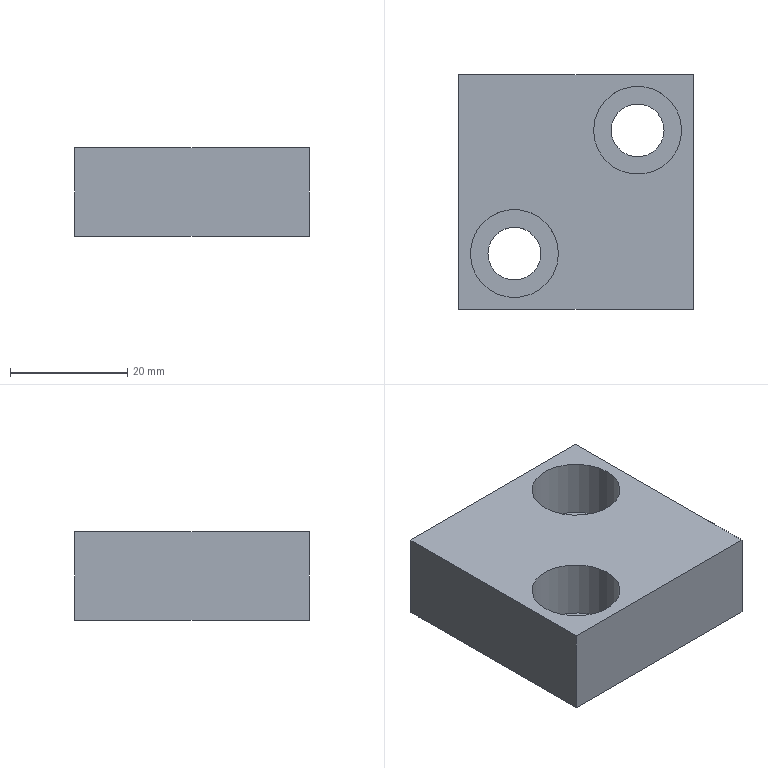Part | NX | features solid 2 | 1 solid | 12 faces | box 40 x 40 x 15 mm | volume 19830 mm3 | plane 8 | cylinder 4 | commonest cylinder face diameters 9 x2 15 x2
STEP:
#1=CARTESIAN_POINT('',(1490.,20.,251.));
#2=VERTEX_POINT('',#1);
#3=CARTESIAN_POINT('',(1490.,20.,266.));
#4=VERTEX_POINT('',#3);
#5=CARTESIAN_POINT('',(1490.,20.,251.));
#6=DIRECTION('',(0.,0.,1.));
#7=VECTOR('',#6,1000.);
#8=LINE('',#5,#7);
#9=EDGE_CURVE('',#2,#4,#8,.T.);
#10=ORIENTED_EDGE('',*,*,#9,.F.);
#11=CARTESIAN_POINT('',(1490.,60.,251.));
#12=VERTEX_POINT('',#11);
#13=CARTESIAN_POINT('',(1490.,60.,251.));
#14=DIRECTION('',(0.,-1.,0.));
#15=VECTOR('',#14,1000.);
#16=LINE('',#13,#15);
#17=EDGE_CURVE('',#12,#2,#16,.T.);
#18=ORIENTED_EDGE('',*,*,#17,.F.);
#19=CARTESIAN_POINT('',(1490.,60.,266.));
#20=VERTEX_POINT('',#19);
#21=CARTESIAN_POINT('',(1490.,60.,251.));
#22=DIRECTION('',(0.,0.,1.));
#23=VECTOR('',#22,1000.);
#24=LINE('',#21,#23);
#25=EDGE_CURVE('',#12,#20,#24,.T.);
#26=ORIENTED_EDGE('',*,*,#25,.T.);
#27=CARTESIAN_POINT('',(1490.,60.,266.));
#28=DIRECTION('',(0.,-1.,0.));
#29=VECTOR('',#28,1000.);
#30=LINE('',#27,#29);
#31=EDGE_CURVE('',#20,#4,#30,.T.);
#32=ORIENTED_EDGE('',*,*,#31,.T.);
#33=EDGE_LOOP('',(#10,#18,#26,#32));
#34=FACE_BOUND('',#33,.T.);
#35=CARTESIAN_POINT('',(1490.,60.,251.));
#36=DIRECTION('',(1.,0.,0.));
#37=DIRECTION('',(0.,0.,1.));
#38=AXIS2_PLACEMENT_3D('',#35,#36,#37);
#39=PLANE('',#38);
#40=ADVANCED_FACE('',(#34),#39,.T.);
#41=CARTESIAN_POINT('',(1450.,20.,251.));
#42=VERTEX_POINT('',#41);
#43=CARTESIAN_POINT('',(1450.,20.,266.));
#44=VERTEX_POINT('',#43);
#45=CARTESIAN_POINT('',(1450.,20.,251.));
#46=DIRECTION('',(0.,0.,1.));
#47=VECTOR('',#46,1000.);
#48=LINE('',#45,#47);
#49=EDGE_CURVE('',#42,#44,#48,.T.);
#50=ORIENTED_EDGE('',*,*,#49,.F.);
#51=CARTESIAN_POINT('',(1490.,20.,251.));
#52=DIRECTION('',(-1.,0.,0.));
#53=VECTOR('',#52,1000.);
#54=LINE('',#51,#53);
#55=EDGE_CURVE('',#2,#42,#54,.T.);
#56=ORIENTED_EDGE('',*,*,#55,.F.);
#57=ORIENTED_EDGE('',*,*,#9,.T.);
#58=CARTESIAN_POINT('',(1490.,20.,266.));
#59=DIRECTION('',(-1.,0.,0.));
#60=VECTOR('',#59,1000.);
#61=LINE('',#58,#60);
#62=EDGE_CURVE('',#4,#44,#61,.T.);
#63=ORIENTED_EDGE('',*,*,#62,.T.);
#64=EDGE_LOOP('',(#50,#56,#57,#63));
#65=FACE_BOUND('',#64,.T.);
#66=CARTESIAN_POINT('',(1490.,20.,251.));
#67=DIRECTION('',(0.,-1.,0.));
#68=DIRECTION('',(0.,0.,-1.));
#69=AXIS2_PLACEMENT_3D('',#66,#67,#68);
#70=PLANE('',#69);
#71=ADVANCED_FACE('',(#65),#70,.T.);
#72=CARTESIAN_POINT('',(1450.,60.,251.));
#73=VERTEX_POINT('',#72);
#74=CARTESIAN_POINT('',(1450.,60.,266.));
#75=VERTEX_POINT('',#74);
#76=CARTESIAN_POINT('',(1450.,60.,251.));
#77=DIRECTION('',(0.,0.,1.));
#78=VECTOR('',#77,1000.);
#79=LINE('',#76,#78);
#80=EDGE_CURVE('',#73,#75,#79,.T.);
#81=ORIENTED_EDGE('',*,*,#80,.F.);
#82=CARTESIAN_POINT('',(1450.,20.,251.));
#83=DIRECTION('',(0.,1.,0.));
#84=VECTOR('',#83,1000.);
#85=LINE('',#82,#84);
#86=EDGE_CURVE('',#42,#73,#85,.T.);
#87=ORIENTED_EDGE('',*,*,#86,.F.);
#88=ORIENTED_EDGE('',*,*,#49,.T.);
#89=CARTESIAN_POINT('',(1450.,20.,266.));
#90=DIRECTION('',(0.,1.,0.));
#91=VECTOR('',#90,1000.);
#92=LINE('',#89,#91);
#93=EDGE_CURVE('',#44,#75,#92,.T.);
#94=ORIENTED_EDGE('',*,*,#93,.T.);
#95=EDGE_LOOP('',(#81,#87,#88,#94));
#96=FACE_BOUND('',#95,.T.);
#97=CARTESIAN_POINT('',(1450.,20.,251.));
#98=DIRECTION('',(-1.,0.,0.));
#99=DIRECTION('',(0.,0.,-1.));
#100=AXIS2_PLACEMENT_3D('',#97,#98,#99);
#101=PLANE('',#100);
#102=ADVANCED_FACE('',(#96),#101,.T.);
#103=CARTESIAN_POINT('',(1464.,29.5,256.));
#104=VERTEX_POINT('',#103);
#105=CARTESIAN_POINT('',(1459.5,29.5,256.));
#106=DIRECTION('',(0.,0.,1.));
#107=DIRECTION('',(1.,0.,0.));
#108=AXIS2_PLACEMENT_3D('',#105,#106,#107);
#109=CIRCLE('',#108,4.5);
#110=EDGE_CURVE('',#104,#104,#109,.F.);
#111=ORIENTED_EDGE('',*,*,#110,.F.);
#112=EDGE_LOOP('',(#111));
#113=FACE_BOUND('',#112,.T.);
#114=CARTESIAN_POINT('',(1455.,29.5,251.));
#115=VERTEX_POINT('',#114);
#116=CARTESIAN_POINT('',(1459.5,29.5,251.));
#117=DIRECTION('',(0.,0.,-1.));
#118=DIRECTION('',(-1.,0.,0.));
#119=AXIS2_PLACEMENT_3D('',#116,#117,#118);
#120=CIRCLE('',#119,4.5);
#121=EDGE_CURVE('',#115,#115,#120,.T.);
#122=ORIENTED_EDGE('',*,*,#121,.T.);
#123=EDGE_LOOP('',(#122));
#124=FACE_BOUND('',#123,.T.);
#125=CARTESIAN_POINT('',(1459.5,29.5,251.));
#126=DIRECTION('',(0.,0.,1.));
#127=DIRECTION('',(-1.,0.,0.));
#128=AXIS2_PLACEMENT_3D('',#125,#126,#127);
#129=CYLINDRICAL_SURFACE('',#128,4.5);
#130=ADVANCED_FACE('',(#113,#124),#129,.F.);
#131=CARTESIAN_POINT('',(1485.,50.5,256.));
#132=VERTEX_POINT('',#131);
#133=CARTESIAN_POINT('',(1480.5,50.5,256.));
#134=DIRECTION('',(0.,0.,1.));
#135=DIRECTION('',(1.,0.,0.));
#136=AXIS2_PLACEMENT_3D('',#133,#134,#135);
#137=CIRCLE('',#136,4.5);
#138=EDGE_CURVE('',#132,#132,#137,.F.);
#139=ORIENTED_EDGE('',*,*,#138,.F.);
#140=EDGE_LOOP('',(#139));
#141=FACE_BOUND('',#140,.T.);
#142=CARTESIAN_POINT('',(1476.,50.5,251.));
#143=VERTEX_POINT('',#142);
#144=CARTESIAN_POINT('',(1480.5,50.5,251.));
#145=DIRECTION('',(0.,0.,-1.));
#146=DIRECTION('',(-1.,0.,0.));
#147=AXIS2_PLACEMENT_3D('',#144,#145,#146);
#148=CIRCLE('',#147,4.5);
#149=EDGE_CURVE('',#143,#143,#148,.T.);
#150=ORIENTED_EDGE('',*,*,#149,.T.);
#151=EDGE_LOOP('',(#150));
#152=FACE_BOUND('',#151,.T.);
#153=CARTESIAN_POINT('',(1480.5,50.5,251.));
#154=DIRECTION('',(0.,0.,1.));
#155=DIRECTION('',(-1.,0.,0.));
#156=AXIS2_PLACEMENT_3D('',#153,#154,#155);
#157=CYLINDRICAL_SURFACE('',#156,4.5);
#158=ADVANCED_FACE('',(#141,#152),#157,.F.);
#159=CARTESIAN_POINT('',(1450.,60.,251.));
#160=DIRECTION('',(1.,0.,0.));
#161=VECTOR('',#160,1000.);
#162=LINE('',#159,#161);
#163=EDGE_CURVE('',#73,#12,#162,.T.);
#164=ORIENTED_EDGE('',*,*,#163,.F.);
#165=ORIENTED_EDGE('',*,*,#80,.T.);
#166=CARTESIAN_POINT('',(1450.,60.,266.));
#167=DIRECTION('',(1.,0.,0.));
#168=VECTOR('',#167,1000.);
#169=LINE('',#166,#168);
#170=EDGE_CURVE('',#75,#20,#169,.T.);
#171=ORIENTED_EDGE('',*,*,#170,.T.);
#172=ORIENTED_EDGE('',*,*,#25,.F.);
#173=EDGE_LOOP('',(#164,#165,#171,#172));
#174=FACE_BOUND('',#173,.T.);
#175=CARTESIAN_POINT('',(1450.,60.,251.));
#176=DIRECTION('',(0.,1.,0.));
#177=DIRECTION('',(1.,0.,0.));
#178=AXIS2_PLACEMENT_3D('',#175,#176,#177);
#179=PLANE('',#178);
#180=ADVANCED_FACE('',(#174),#179,.T.);
#181=ORIENTED_EDGE('',*,*,#149,.F.);
#182=EDGE_LOOP('',(#181));
#183=FACE_BOUND('',#182,.T.);
#184=ORIENTED_EDGE('',*,*,#121,.F.);
#185=EDGE_LOOP('',(#184));
#186=FACE_BOUND('',#185,.T.);
#187=ORIENTED_EDGE('',*,*,#17,.T.);
#188=ORIENTED_EDGE('',*,*,#55,.T.);
#189=ORIENTED_EDGE('',*,*,#86,.T.);
#190=ORIENTED_EDGE('',*,*,#163,.T.);
#191=EDGE_LOOP('',(#187,#188,#189,#190));
#192=FACE_BOUND('',#191,.T.);
#193=CARTESIAN_POINT('',(1490.,20.,251.));
#194=DIRECTION('',(0.,0.,1.));
#195=DIRECTION('',(-1.,0.,0.));
#196=AXIS2_PLACEMENT_3D('',#193,#194,#195);
#197=PLANE('',#196);
#198=ADVANCED_FACE('',(#183,#186,#192),#197,.F.);
#199=CARTESIAN_POINT('',(1467.,29.5,266.));
#200=VERTEX_POINT('',#199);
#201=CARTESIAN_POINT('',(1459.5,29.5,266.));
#202=DIRECTION('',(0.,0.,1.));
#203=DIRECTION('',(1.,0.,0.));
#204=AXIS2_PLACEMENT_3D('',#201,#202,#203);
#205=CIRCLE('',#204,7.5);
#206=EDGE_CURVE('',#200,#200,#205,.T.);
#207=ORIENTED_EDGE('',*,*,#206,.F.);
#208=EDGE_LOOP('',(#207));
#209=FACE_BOUND('',#208,.T.);
#210=CARTESIAN_POINT('',(1488.,50.5,266.));
#211=VERTEX_POINT('',#210);
#212=CARTESIAN_POINT('',(1480.5,50.5,266.));
#213=DIRECTION('',(0.,0.,1.));
#214=DIRECTION('',(1.,0.,0.));
#215=AXIS2_PLACEMENT_3D('',#212,#213,#214);
#216=CIRCLE('',#215,7.5);
#217=EDGE_CURVE('',#211,#211,#216,.T.);
#218=ORIENTED_EDGE('',*,*,#217,.F.);
#219=EDGE_LOOP('',(#218));
#220=FACE_BOUND('',#219,.T.);
#221=ORIENTED_EDGE('',*,*,#31,.F.);
#222=ORIENTED_EDGE('',*,*,#170,.F.);
#223=ORIENTED_EDGE('',*,*,#93,.F.);
#224=ORIENTED_EDGE('',*,*,#62,.F.);
#225=EDGE_LOOP('',(#221,#222,#223,#224));
#226=FACE_BOUND('',#225,.T.);
#227=CARTESIAN_POINT('',(1490.,20.,266.));
#228=DIRECTION('',(0.,0.,1.));
#229=DIRECTION('',(-1.,0.,0.));
#230=AXIS2_PLACEMENT_3D('',#227,#228,#229);
#231=PLANE('',#230);
#232=ADVANCED_FACE('',(#209,#220,#226),#231,.T.);
#233=CARTESIAN_POINT('',(1488.,50.5,256.));
#234=VERTEX_POINT('',#233);
#235=CARTESIAN_POINT('',(1480.5,50.5,256.));
#236=DIRECTION('',(0.,0.,1.));
#237=DIRECTION('',(1.,0.,0.));
#238=AXIS2_PLACEMENT_3D('',#235,#236,#237);
#239=CIRCLE('',#238,7.5);
#240=EDGE_CURVE('',#234,#234,#239,.T.);
#241=ORIENTED_EDGE('',*,*,#240,.T.);
#242=EDGE_LOOP('',(#241));
#243=FACE_BOUND('',#242,.T.);
#244=ORIENTED_EDGE('',*,*,#138,.T.);
#245=EDGE_LOOP('',(#244));
#246=FACE_BOUND('',#245,.T.);
#247=CARTESIAN_POINT('',(1480.5,50.5,256.));
#248=DIRECTION('',(0.,0.,-1.));
#249=DIRECTION('',(1.,0.,0.));
#250=AXIS2_PLACEMENT_3D('',#247,#248,#249);
#251=PLANE('',#250);
#252=ADVANCED_FACE('',(#243,#246),#251,.F.);
#253=ORIENTED_EDGE('',*,*,#240,.F.);
#254=EDGE_LOOP('',(#253));
#255=FACE_BOUND('',#254,.T.);
#256=ORIENTED_EDGE('',*,*,#217,.T.);
#257=EDGE_LOOP('',(#256));
#258=FACE_BOUND('',#257,.T.);
#259=CARTESIAN_POINT('',(1480.5,50.5,266.));
#260=DIRECTION('',(0.,0.,-1.));
#261=DIRECTION('',(1.,0.,0.));
#262=AXIS2_PLACEMENT_3D('',#259,#260,#261);
#263=CYLINDRICAL_SURFACE('',#262,7.5);
#264=ADVANCED_FACE('',(#255,#258),#263,.F.);
#265=CARTESIAN_POINT('',(1467.,29.5,256.));
#266=VERTEX_POINT('',#265);
#267=CARTESIAN_POINT('',(1459.5,29.5,256.));
#268=DIRECTION('',(0.,0.,1.));
#269=DIRECTION('',(1.,0.,0.));
#270=AXIS2_PLACEMENT_3D('',#267,#268,#269);
#271=CIRCLE('',#270,7.5);
#272=EDGE_CURVE('',#266,#266,#271,.T.);
#273=ORIENTED_EDGE('',*,*,#272,.T.);
#274=EDGE_LOOP('',(#273));
#275=FACE_BOUND('',#274,.T.);
#276=ORIENTED_EDGE('',*,*,#110,.T.);
#277=EDGE_LOOP('',(#276));
#278=FACE_BOUND('',#277,.T.);
#279=CARTESIAN_POINT('',(1459.5,29.5,256.));
#280=DIRECTION('',(0.,0.,-1.));
#281=DIRECTION('',(1.,0.,0.));
#282=AXIS2_PLACEMENT_3D('',#279,#280,#281);
#283=PLANE('',#282);
#284=ADVANCED_FACE('',(#275,#278),#283,.F.);
#285=ORIENTED_EDGE('',*,*,#272,.F.);
#286=EDGE_LOOP('',(#285));
#287=FACE_BOUND('',#286,.T.);
#288=ORIENTED_EDGE('',*,*,#206,.T.);
#289=EDGE_LOOP('',(#288));
#290=FACE_BOUND('',#289,.T.);
#291=CARTESIAN_POINT('',(1459.5,29.5,266.));
#292=DIRECTION('',(0.,0.,-1.));
#293=DIRECTION('',(1.,0.,0.));
#294=AXIS2_PLACEMENT_3D('',#291,#292,#293);
#295=CYLINDRICAL_SURFACE('',#294,7.5);
#296=ADVANCED_FACE('',(#287,#290),#295,.F.);
#297=CLOSED_SHELL('',(#40,#71,#102,#130,#158,#180,#198,#232,#252,#264,#284,#296));
#298=MANIFOLD_SOLID_BREP('',#297);
#299=(LENGTH_UNIT()NAMED_UNIT(*)SI_UNIT(.MILLI.,.METRE.));
#300=UNCERTAINTY_MEASURE_WITH_UNIT(LENGTH_MEASURE(0.00001),#299,'','');
#301=(NAMED_UNIT(*)PLANE_ANGLE_UNIT()SI_UNIT($,.RADIAN.));
#302=(NAMED_UNIT(*)SI_UNIT($,.STERADIAN.)SOLID_ANGLE_UNIT());
#303=(GEOMETRIC_REPRESENTATION_CONTEXT(3)GLOBAL_UNCERTAINTY_ASSIGNED_CONTEXT((#300))GLOBAL_UNIT_ASSIGNED_CONTEXT((#299,#301,#302))REPRESENTATION_CONTEXT('',''));
#304=ADVANCED_BREP_SHAPE_REPRESENTATION('',(#298),#303);